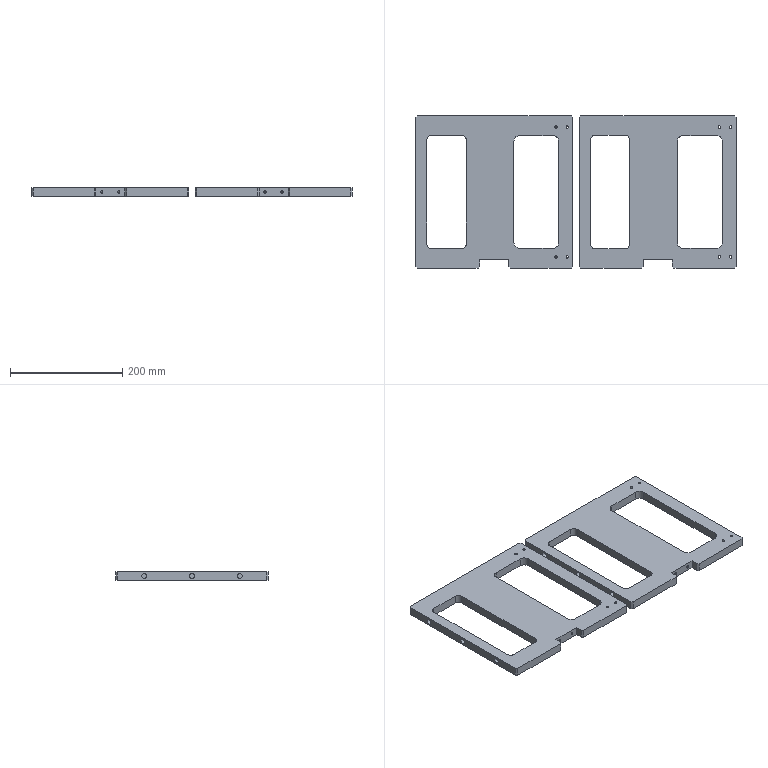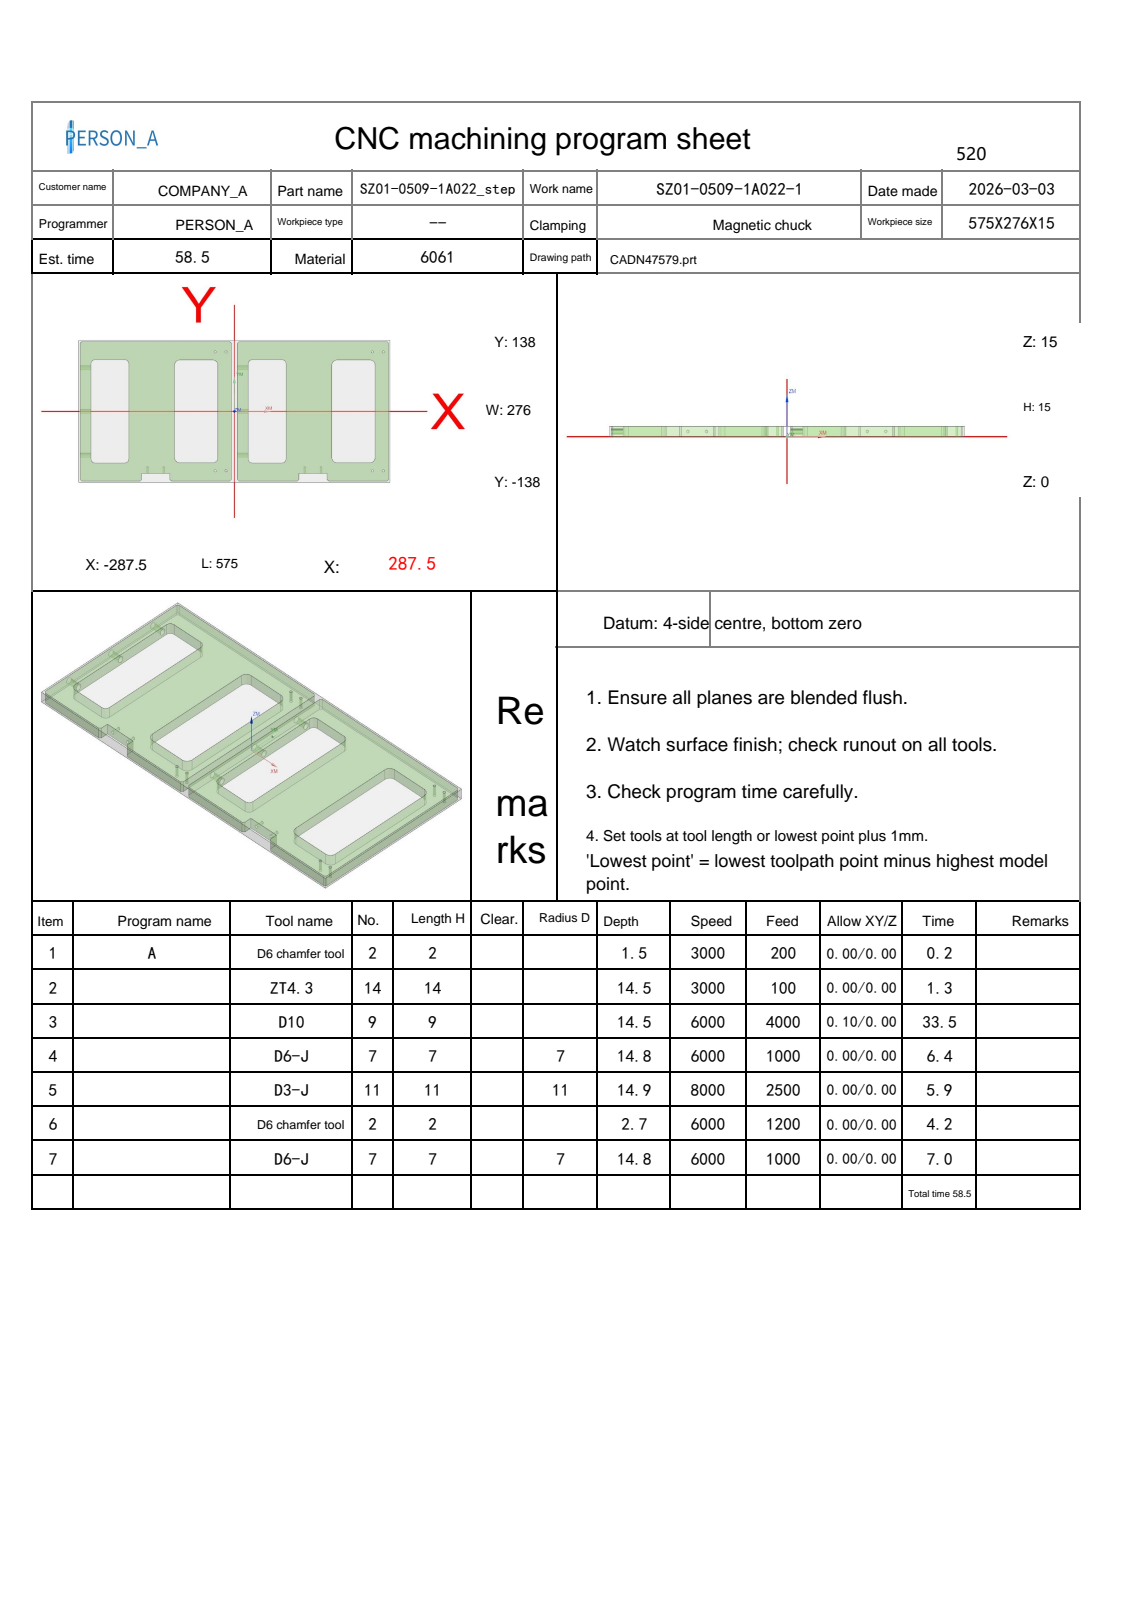NC program | NX | posted by the shop | part box 570 x 271 x 15 mm
Lines 2745 to 2981 of 10286:
N4 T07 M06
(D6-J  D=6. R=0. H=07 ce=0.00 di=0.00)
(D.N=07 MAX_Z=45. MIN_Z=0.2 Time=6.49M)
G00 G90 G54 X-34.784 Y-91. M03 S6000
G43 H07 Z45.
M08
Z8.25
G01 Z7.75 F1000.
G41 D07
X-34.5
G03 X-33.5 Y-90. I0.0 J1.
G01 Y90.
G03 X-40.5 Y97. I-7. J0.0
G01 X-100.5
G03 X-107.5 Y90. I0.0 J-7.
G01 Y-90.
G03 X-100.5 Y-97. I7. J0.0
G01 X-40.5
G03 X-33.5 Y-90. I0.0 J7.
G01 Y-89.5
G03 X-34.5 Y-88.5 I-1. J0.0
G01 G40 X-34.7
Z8.25
G00 X-34.784 Y-91.
Z1.
G01 Z.5
G41 D07
X-34.5
G03 X-33.5 Y-90. I0.0 J1.
G01 Y90.
G03 X-40.5 Y97. I-7. J0.0
G01 X-100.5
G03 X-107.5 Y90. I0.0 J-7.
G01 Y-90.
G03 X-100.5 Y-97. I7. J0.0
G01 X-40.5
G03 X-33.5 Y-90. I0.0 J7.
G01 Y-89.5
G03 X-34.5 Y-88.5 I-1. J0.0
G01 G40 X-34.7
Z1.
G00 Z45.
X255.716 Y-91.
Z8.25
G01 Z7.75
G41 D07
X256.
G03 X257. Y-90. I0.0 J1.
G01 Y90.
G03 X250. Y97. I-7. J0.0
G01 X190.
G03 X183. Y90. I0.0 J-7.
G01 Y-90.
G03 X190. Y-97. I7. J0.0
G01 X250.
G03 X257. Y-90. I0.0 J7.
G01 Y-89.5
G03 X256. Y-88.5 I-1. J0.0
G01 G40 X255.8
Z8.25
G00 X255.716 Y-91.
Z1.
G01 Z.5
G41 D07
X256.
G03 X257. Y-90. I0.0 J1.
G01 Y90.
G03 X250. Y97. I-7. J0.0
G01 X190.
G03 X183. Y90. I0.0 J-7.
G01 Y-90.
G03 X190. Y-97. I7. J0.0
G01 X250.
G03 X257. Y-90. I0.0 J7.
G01 Y-89.5
G03 X256. Y-88.5 I-1. J0.0
G01 G40 X255.8
Z1.
G00 Z45.
G00 G90 X-260.673 Y93.5 M03 S6000
Z45.
Z8.25
G01 Z7.75 F1000.
G41 D07
X-261.
G03 X-262. Y92.5 I0.0 J-1.
G01 Y-92.5
G03 X-257. Y-97.5 I5. J0.0
G01 X-203.
G03 X-198. Y-92.5 I0.0 J5.
G01 Y92.5
G03 X-203. Y97.5 I-5. J0.0
G01 X-257.
G03 X-262. Y92.5 I0.0 J-5.
G01 Y92.
G03 X-261. Y91. I1. J0.0
G01 G40 X-260.8
Z8.25
G00 X-260.673 Y93.5
Z1.
G01 Z.5
G41 D07
X-261.
G03 X-262. Y92.5 I0.0 J-1.
G01 Y-92.5
G03 X-257. Y-97.5 I5. J0.0
G01 X-203.
G03 X-198. Y-92.5 I0.0 J5.
G01 Y92.5
G03 X-203. Y97.5 I-5. J0.0
G01 X-257.
G03 X-262. Y92.5 I0.0 J-5.
G01 Y92.
G03 X-261. Y91. I1. J0.0
G01 G40 X-260.8
Z1.
G00 Z45.
X29.827 Y93.5
Z8.25
G01 Z7.75
G41 D07
X29.5
G03 X28.5 Y92.5 I0.0 J-1.
G01 Y-92.5
G03 X33.5 Y-97.5 I5. J0.0
G01 X87.5
G03 X92.5 Y-92.5 I0.0 J5.
G01 Y92.5
G03 X87.5 Y97.5 I-5. J0.0
G01 X33.5
G03 X28.5 Y92.5 I0.0 J-5.
G01 Y92.
G03 X29.5 Y91. I1. J0.0
G01 G40 X29.7
Z8.25
G00 X29.827 Y93.5
Z1.
G01 Z.5
G41 D07
X29.5
G03 X28.5 Y92.5 I0.0 J-1.
G01 Y-92.5
G03 X33.5 Y-97.5 I5. J0.0
G01 X87.5
G03 X92.5 Y-92.5 I0.0 J5.
G01 Y92.5
G03 X87.5 Y97.5 I-5. J0.0
G01 X33.5
G03 X28.5 Y92.5 I0.0 J-5.
G01 Y92.
G03 X29.5 Y91. I1. J0.0
G01 G40 X29.7
Z1.
G00 Z45.
G00 G90 X-34.684 Y-91. M03 S6000
Z45.
Z.7
G01 Z.2 F1000.
G41 D07
X-34.5
G03 X-33.5 Y-90. I0.0 J1.
G01 Y90.
G03 X-40.5 Y97. I-7. J0.0
G01 X-100.5
G03 X-107.5 Y90. I0.0 J-7.
G01 Y-90.
G03 X-100.5 Y-97. I7. J0.0
G01 X-40.5
G03 X-33.5 Y-90. I0.0 J7.
G01 Y-89.5
G03 X-34.5 Y-88.5 I-1. J0.0
G01 G40 X-34.6
Z.7
G00 Z45.
X255.816 Y-91.
Z.7
G01 Z.2
G41 D07
X256.
G03 X257. Y-90. I0.0 J1.
G01 Y90.
G03 X250. Y97. I-7. J0.0
G01 X190.
G03 X183. Y90. I0.0 J-7.
G01 Y-90.
G03 X190. Y-97. I7. J0.0
G01 X250.
G03 X257. Y-90. I0.0 J7.
G01 Y-89.5
G03 X256. Y-88.5 I-1. J0.0
G01 G40 X255.9
Z.7
G00 Z45.
G00 G90 X-260.773 Y93.5 M03 S6000
Z45.
Z.7
G01 Z.2 F1000.
G41 D07
X-261.
G03 X-262. Y92.5 I0.0 J-1.
G01 Y-92.5
G03 X-257. Y-97.5 I5. J0.0
G01 X-203.
G03 X-198. Y-92.5 I0.0 J5.
G01 Y92.5
G03 X-203. Y97.5 I-5. J0.0
G01 X-257.
G03 X-262. Y92.5 I0.0 J-5.
G01 Y92.
G03 X-261. Y91. I1. J0.0
G01 G40 X-260.9
Z.7
G00 Z45.
X29.727 Y93.5
Z.7
G01 Z.2
G41 D07
X29.5
G03 X28.5 Y92.5 I0.0 J-1.
G01 Y-92.5
G03 X33.5 Y-97.5 I5. J0.0
G01 X87.5
G03 X92.5 Y-92.5 I0.0 J5.
G01 Y92.5
G03 X87.5 Y97.5 I-5. J0.0
G01 X33.5
G03 X28.5 Y92.5 I0.0 J-5.
G01 Y92.
G03 X29.5 Y91. I1. J0.0
G01 G40 X29.6
Z.7
G00 Z45.
G91 G28 Z0.0
M05
M09
G91 G28 Z0.0
M01